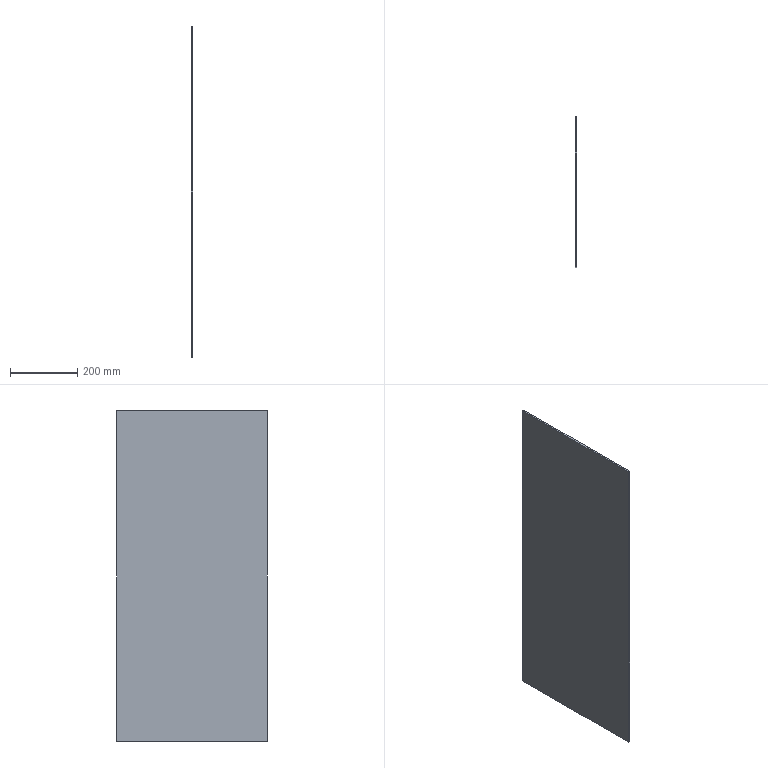Part | SolidWorks | features Chamfer 1, ICE 1 | 1 solid | 10 faces | box 5 x 448 x 985 mm | volume 2206390 mm3 | plane 10
STEP:
#1=CARTESIAN_POINT('',(5.,-223.,-492.5));
#2=VERTEX_POINT('',#1);
#3=CARTESIAN_POINT('',(5.,223.,-492.5));
#4=VERTEX_POINT('',#3);
#5=CARTESIAN_POINT('',(5.,224.,-492.5));
#6=DIRECTION('',(0.,1.,0.));
#7=VECTOR('',#6,1000.);
#8=LINE('',#5,#7);
#9=EDGE_CURVE('',#2,#4,#8,.T.);
#10=ORIENTED_EDGE('',*,*,#9,.F.);
#11=CARTESIAN_POINT('',(0.,-223.,-492.5));
#12=VERTEX_POINT('',#11);
#13=CARTESIAN_POINT('',(5.,-223.,-492.5));
#14=DIRECTION('',(-1.,0.,0.));
#15=VECTOR('',#14,1000.);
#16=LINE('',#13,#15);
#17=EDGE_CURVE('',#2,#12,#16,.T.);
#18=ORIENTED_EDGE('',*,*,#17,.T.);
#19=CARTESIAN_POINT('',(0.,223.,-492.5));
#20=VERTEX_POINT('',#19);
#21=CARTESIAN_POINT('',(0.,224.,-492.5));
#22=DIRECTION('',(0.,1.,0.));
#23=VECTOR('',#22,1000.);
#24=LINE('',#21,#23);
#25=EDGE_CURVE('',#12,#20,#24,.T.);
#26=ORIENTED_EDGE('',*,*,#25,.T.);
#27=CARTESIAN_POINT('',(5.,223.,-492.5));
#28=DIRECTION('',(1.,0.,0.));
#29=VECTOR('',#28,1000.);
#30=LINE('',#27,#29);
#31=EDGE_CURVE('',#20,#4,#30,.T.);
#32=ORIENTED_EDGE('',*,*,#31,.T.);
#33=EDGE_LOOP('',(#10,#18,#26,#32));
#34=FACE_OUTER_BOUND('',#33,.T.);
#35=CARTESIAN_POINT('',(5.,224.,-492.5));
#36=DIRECTION('',(0.,0.,1.));
#37=DIRECTION('',(1.,0.,0.));
#38=AXIS2_PLACEMENT_3D('',#35,#36,#37);
#39=PLANE('',#38);
#40=ADVANCED_FACE('',(#34),#39,.F.);
#41=CARTESIAN_POINT('',(0.,224.,-491.5));
#42=VERTEX_POINT('',#41);
#43=CARTESIAN_POINT('',(0.,224.,491.5));
#44=VERTEX_POINT('',#43);
#45=CARTESIAN_POINT('',(0.,224.,492.5));
#46=DIRECTION('',(0.,0.,1.));
#47=VECTOR('',#46,1000.);
#48=LINE('',#45,#47);
#49=EDGE_CURVE('',#42,#44,#48,.T.);
#50=ORIENTED_EDGE('',*,*,#49,.T.);
#51=CARTESIAN_POINT('',(5.,224.,491.5));
#52=VERTEX_POINT('',#51);
#53=CARTESIAN_POINT('',(5.,224.,491.5));
#54=DIRECTION('',(1.,0.,0.));
#55=VECTOR('',#54,1000.);
#56=LINE('',#53,#55);
#57=EDGE_CURVE('',#44,#52,#56,.T.);
#58=ORIENTED_EDGE('',*,*,#57,.T.);
#59=CARTESIAN_POINT('',(5.,224.,-491.5));
#60=VERTEX_POINT('',#59);
#61=CARTESIAN_POINT('',(5.,224.,492.5));
#62=DIRECTION('',(0.,0.,1.));
#63=VECTOR('',#62,1000.);
#64=LINE('',#61,#63);
#65=EDGE_CURVE('',#60,#52,#64,.T.);
#66=ORIENTED_EDGE('',*,*,#65,.F.);
#67=CARTESIAN_POINT('',(5.,224.,-491.5));
#68=DIRECTION('',(-1.,0.,0.));
#69=VECTOR('',#68,1000.);
#70=LINE('',#67,#69);
#71=EDGE_CURVE('',#60,#42,#70,.T.);
#72=ORIENTED_EDGE('',*,*,#71,.T.);
#73=EDGE_LOOP('',(#50,#58,#66,#72));
#74=FACE_OUTER_BOUND('',#73,.T.);
#75=CARTESIAN_POINT('',(5.,224.,492.5));
#76=DIRECTION('',(0.,-1.,0.));
#77=DIRECTION('',(0.,0.,-1.));
#78=AXIS2_PLACEMENT_3D('',#75,#76,#77);
#79=PLANE('',#78);
#80=ADVANCED_FACE('',(#74),#79,.F.);
#81=CARTESIAN_POINT('',(5.,223.,492.5));
#82=VERTEX_POINT('',#81);
#83=CARTESIAN_POINT('',(5.,-223.,492.5));
#84=VERTEX_POINT('',#83);
#85=CARTESIAN_POINT('',(5.,224.,492.5));
#86=DIRECTION('',(0.,-1.,0.));
#87=VECTOR('',#86,1000.);
#88=LINE('',#85,#87);
#89=EDGE_CURVE('',#82,#84,#88,.T.);
#90=ORIENTED_EDGE('',*,*,#89,.F.);
#91=CARTESIAN_POINT('',(0.,223.,492.5));
#92=VERTEX_POINT('',#91);
#93=CARTESIAN_POINT('',(5.,223.,492.5));
#94=DIRECTION('',(-1.,0.,0.));
#95=VECTOR('',#94,1000.);
#96=LINE('',#93,#95);
#97=EDGE_CURVE('',#82,#92,#96,.T.);
#98=ORIENTED_EDGE('',*,*,#97,.T.);
#99=CARTESIAN_POINT('',(0.,-223.,492.5));
#100=VERTEX_POINT('',#99);
#101=CARTESIAN_POINT('',(0.,224.,492.5));
#102=DIRECTION('',(0.,-1.,0.));
#103=VECTOR('',#102,1000.);
#104=LINE('',#101,#103);
#105=EDGE_CURVE('',#92,#100,#104,.T.);
#106=ORIENTED_EDGE('',*,*,#105,.T.);
#107=CARTESIAN_POINT('',(5.,-223.,492.5));
#108=DIRECTION('',(1.,0.,0.));
#109=VECTOR('',#108,1000.);
#110=LINE('',#107,#109);
#111=EDGE_CURVE('',#100,#84,#110,.T.);
#112=ORIENTED_EDGE('',*,*,#111,.T.);
#113=EDGE_LOOP('',(#90,#98,#106,#112));
#114=FACE_OUTER_BOUND('',#113,.T.);
#115=CARTESIAN_POINT('',(5.,224.,492.5));
#116=DIRECTION('',(0.,0.,-1.));
#117=DIRECTION('',(-1.,0.,0.));
#118=AXIS2_PLACEMENT_3D('',#115,#116,#117);
#119=PLANE('',#118);
#120=ADVANCED_FACE('',(#114),#119,.F.);
#121=CARTESIAN_POINT('',(5.,-224.,491.5));
#122=VERTEX_POINT('',#121);
#123=CARTESIAN_POINT('',(5.,-224.,-491.5));
#124=VERTEX_POINT('',#123);
#125=CARTESIAN_POINT('',(5.,-224.,492.5));
#126=DIRECTION('',(0.,0.,-1.));
#127=VECTOR('',#126,1000.);
#128=LINE('',#125,#127);
#129=EDGE_CURVE('',#122,#124,#128,.T.);
#130=ORIENTED_EDGE('',*,*,#129,.F.);
#131=CARTESIAN_POINT('',(0.,-224.,491.5));
#132=VERTEX_POINT('',#131);
#133=CARTESIAN_POINT('',(5.,-224.,491.5));
#134=DIRECTION('',(-1.,0.,0.));
#135=VECTOR('',#134,1000.);
#136=LINE('',#133,#135);
#137=EDGE_CURVE('',#122,#132,#136,.T.);
#138=ORIENTED_EDGE('',*,*,#137,.T.);
#139=CARTESIAN_POINT('',(0.,-224.,-491.5));
#140=VERTEX_POINT('',#139);
#141=CARTESIAN_POINT('',(0.,-224.,492.5));
#142=DIRECTION('',(0.,0.,-1.));
#143=VECTOR('',#142,1000.);
#144=LINE('',#141,#143);
#145=EDGE_CURVE('',#132,#140,#144,.T.);
#146=ORIENTED_EDGE('',*,*,#145,.T.);
#147=CARTESIAN_POINT('',(5.,-224.,-491.5));
#148=DIRECTION('',(1.,0.,0.));
#149=VECTOR('',#148,1000.);
#150=LINE('',#147,#149);
#151=EDGE_CURVE('',#140,#124,#150,.T.);
#152=ORIENTED_EDGE('',*,*,#151,.T.);
#153=EDGE_LOOP('',(#130,#138,#146,#152));
#154=FACE_OUTER_BOUND('',#153,.T.);
#155=CARTESIAN_POINT('',(5.,-224.,492.5));
#156=DIRECTION('',(0.,1.,0.));
#157=DIRECTION('',(0.,0.,1.));
#158=AXIS2_PLACEMENT_3D('',#155,#156,#157);
#159=PLANE('',#158);
#160=ADVANCED_FACE('',(#154),#159,.F.);
#161=ORIENTED_EDGE('',*,*,#65,.T.);
#162=CARTESIAN_POINT('',(5.,357.75,357.75));
#163=DIRECTION('',(0.,-0.7071,0.7071));
#164=VECTOR('',#163,1000.);
#165=LINE('',#162,#164);
#166=EDGE_CURVE('',#52,#82,#165,.T.);
#167=ORIENTED_EDGE('',*,*,#166,.T.);
#168=ORIENTED_EDGE('',*,*,#89,.T.);
#169=CARTESIAN_POINT('',(5.,-357.75,357.75));
#170=DIRECTION('',(0.,-0.7071,-0.7071));
#171=VECTOR('',#170,1000.);
#172=LINE('',#169,#171);
#173=EDGE_CURVE('',#84,#122,#172,.T.);
#174=ORIENTED_EDGE('',*,*,#173,.T.);
#175=ORIENTED_EDGE('',*,*,#129,.T.);
#176=CARTESIAN_POINT('',(5.,-357.75,-357.75));
#177=DIRECTION('',(0.,0.7071,-0.7071));
#178=VECTOR('',#177,1000.);
#179=LINE('',#176,#178);
#180=EDGE_CURVE('',#124,#2,#179,.T.);
#181=ORIENTED_EDGE('',*,*,#180,.T.);
#182=ORIENTED_EDGE('',*,*,#9,.T.);
#183=CARTESIAN_POINT('',(5.,357.75,-357.75));
#184=DIRECTION('',(0.,0.7071,0.7071));
#185=VECTOR('',#184,1000.);
#186=LINE('',#183,#185);
#187=EDGE_CURVE('',#4,#60,#186,.T.);
#188=ORIENTED_EDGE('',*,*,#187,.T.);
#189=EDGE_LOOP('',(#161,#167,#168,#174,#175,#181,#182,#188));
#190=FACE_OUTER_BOUND('',#189,.T.);
#191=CARTESIAN_POINT('',(5.,0.,0.));
#192=DIRECTION('',(1.,0.,0.));
#193=DIRECTION('',(0.,0.,-1.));
#194=AXIS2_PLACEMENT_3D('',#191,#192,#193);
#195=PLANE('',#194);
#196=ADVANCED_FACE('',(#190),#195,.T.);
#197=ORIENTED_EDGE('',*,*,#105,.F.);
#198=CARTESIAN_POINT('',(0.,223.,492.5));
#199=DIRECTION('',(0.,0.7071,-0.7071));
#200=VECTOR('',#199,1000.);
#201=LINE('',#198,#200);
#202=EDGE_CURVE('',#92,#44,#201,.T.);
#203=ORIENTED_EDGE('',*,*,#202,.T.);
#204=ORIENTED_EDGE('',*,*,#49,.F.);
#205=CARTESIAN_POINT('',(0.,224.,-491.5));
#206=DIRECTION('',(0.,-0.7071,-0.7071));
#207=VECTOR('',#206,1000.);
#208=LINE('',#205,#207);
#209=EDGE_CURVE('',#42,#20,#208,.T.);
#210=ORIENTED_EDGE('',*,*,#209,.T.);
#211=ORIENTED_EDGE('',*,*,#25,.F.);
#212=CARTESIAN_POINT('',(0.,-223.,-492.5));
#213=DIRECTION('',(0.,-0.7071,0.7071));
#214=VECTOR('',#213,1000.);
#215=LINE('',#212,#214);
#216=EDGE_CURVE('',#12,#140,#215,.T.);
#217=ORIENTED_EDGE('',*,*,#216,.T.);
#218=ORIENTED_EDGE('',*,*,#145,.F.);
#219=CARTESIAN_POINT('',(0.,-224.,491.5));
#220=DIRECTION('',(0.,0.7071,0.7071));
#221=VECTOR('',#220,1000.);
#222=LINE('',#219,#221);
#223=EDGE_CURVE('',#132,#100,#222,.T.);
#224=ORIENTED_EDGE('',*,*,#223,.T.);
#225=EDGE_LOOP('',(#197,#203,#204,#210,#211,#217,#218,#224));
#226=FACE_OUTER_BOUND('',#225,.T.);
#227=CARTESIAN_POINT('',(0.,0.,0.));
#228=DIRECTION('',(1.,0.,0.));
#229=DIRECTION('',(0.,0.,-1.));
#230=AXIS2_PLACEMENT_3D('',#227,#228,#229);
#231=PLANE('',#230);
#232=ADVANCED_FACE('',(#226),#231,.F.);
#233=ORIENTED_EDGE('',*,*,#166,.F.);
#234=ORIENTED_EDGE('',*,*,#57,.F.);
#235=ORIENTED_EDGE('',*,*,#202,.F.);
#236=ORIENTED_EDGE('',*,*,#97,.F.);
#237=EDGE_LOOP('',(#233,#234,#235,#236));
#238=FACE_OUTER_BOUND('',#237,.T.);
#239=CARTESIAN_POINT('',(5.,223.,492.5));
#240=DIRECTION('',(0.,-0.7071,-0.7071));
#241=DIRECTION('',(-1.,0.,0.));
#242=AXIS2_PLACEMENT_3D('',#239,#240,#241);
#243=PLANE('',#242);
#244=ADVANCED_FACE('',(#238),#243,.F.);
#245=ORIENTED_EDGE('',*,*,#173,.F.);
#246=ORIENTED_EDGE('',*,*,#111,.F.);
#247=ORIENTED_EDGE('',*,*,#223,.F.);
#248=ORIENTED_EDGE('',*,*,#137,.F.);
#249=EDGE_LOOP('',(#245,#246,#247,#248));
#250=FACE_OUTER_BOUND('',#249,.T.);
#251=CARTESIAN_POINT('',(5.,-224.,491.5));
#252=DIRECTION('',(0.,0.7071,-0.7071));
#253=DIRECTION('',(-1.,0.,0.));
#254=AXIS2_PLACEMENT_3D('',#251,#252,#253);
#255=PLANE('',#254);
#256=ADVANCED_FACE('',(#250),#255,.F.);
#257=ORIENTED_EDGE('',*,*,#180,.F.);
#258=ORIENTED_EDGE('',*,*,#151,.F.);
#259=ORIENTED_EDGE('',*,*,#216,.F.);
#260=ORIENTED_EDGE('',*,*,#17,.F.);
#261=EDGE_LOOP('',(#257,#258,#259,#260));
#262=FACE_OUTER_BOUND('',#261,.T.);
#263=CARTESIAN_POINT('',(5.,-223.,-492.5));
#264=DIRECTION('',(0.,0.7071,0.7071));
#265=DIRECTION('',(-1.,0.,0.));
#266=AXIS2_PLACEMENT_3D('',#263,#264,#265);
#267=PLANE('',#266);
#268=ADVANCED_FACE('',(#262),#267,.F.);
#269=ORIENTED_EDGE('',*,*,#187,.F.);
#270=ORIENTED_EDGE('',*,*,#31,.F.);
#271=ORIENTED_EDGE('',*,*,#209,.F.);
#272=ORIENTED_EDGE('',*,*,#71,.F.);
#273=EDGE_LOOP('',(#269,#270,#271,#272));
#274=FACE_OUTER_BOUND('',#273,.T.);
#275=CARTESIAN_POINT('',(5.,224.,-491.5));
#276=DIRECTION('',(0.,-0.7071,0.7071));
#277=DIRECTION('',(-1.,0.,0.));
#278=AXIS2_PLACEMENT_3D('',#275,#276,#277);
#279=PLANE('',#278);
#280=ADVANCED_FACE('',(#274),#279,.F.);
#281=CLOSED_SHELL('',(#40,#80,#120,#160,#196,#232,#244,#256,#268,#280));
#282=MANIFOLD_SOLID_BREP('',#281);
#283=CARTESIAN_POINT('',(0.,0.,0.));
#284=DIRECTION('',(0.,0.,1.));
#285=DIRECTION('',(1.,0.,0.));
#286=AXIS2_PLACEMENT_3D('',#283,#284,#285);
#287=(LENGTH_UNIT()NAMED_UNIT(*)SI_UNIT(.MILLI.,.METRE.));
#288=UNCERTAINTY_MEASURE_WITH_UNIT(LENGTH_MEASURE(0.00001),#287,'','');
#289=(NAMED_UNIT(*)PLANE_ANGLE_UNIT()SI_UNIT($,.RADIAN.));
#290=(NAMED_UNIT(*)SI_UNIT($,.STERADIAN.)SOLID_ANGLE_UNIT());
#291=(GEOMETRIC_REPRESENTATION_CONTEXT(3)GLOBAL_UNCERTAINTY_ASSIGNED_CONTEXT((#288))GLOBAL_UNIT_ASSIGNED_CONTEXT((#287,#289,#290))REPRESENTATION_CONTEXT('',''));
#292=ADVANCED_BREP_SHAPE_REPRESENTATION('',(#282,#286),#291);